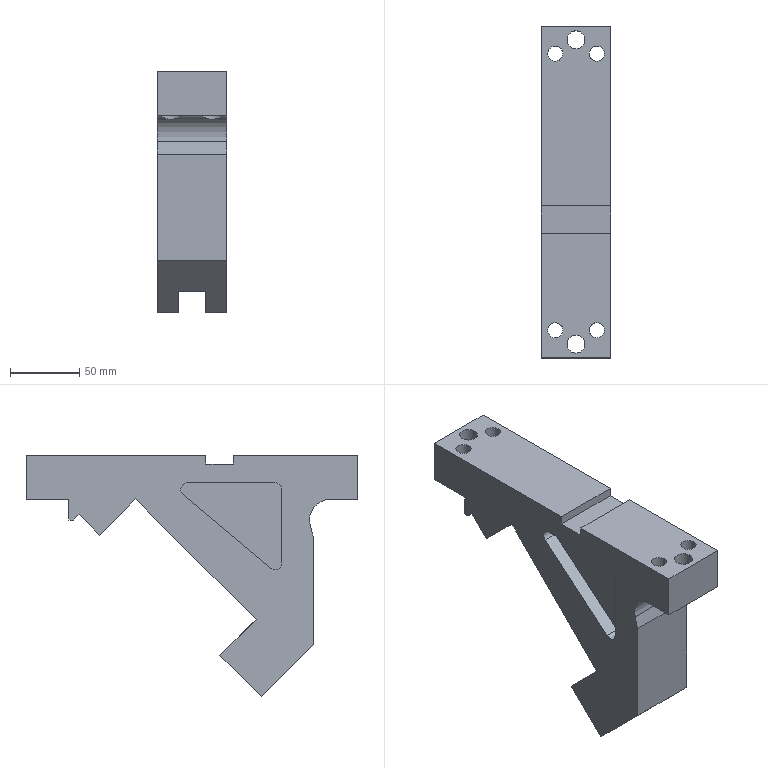Part | NX | features solid 2 | 1 solid | 59 faces | box 50 x 240 x 174.933 mm | volume 786576 mm3 | plane 42 | cylinder 17 | commonest cylinder face diameters 10 x6 11 x4 17.5 x4 13 x2 30 x1